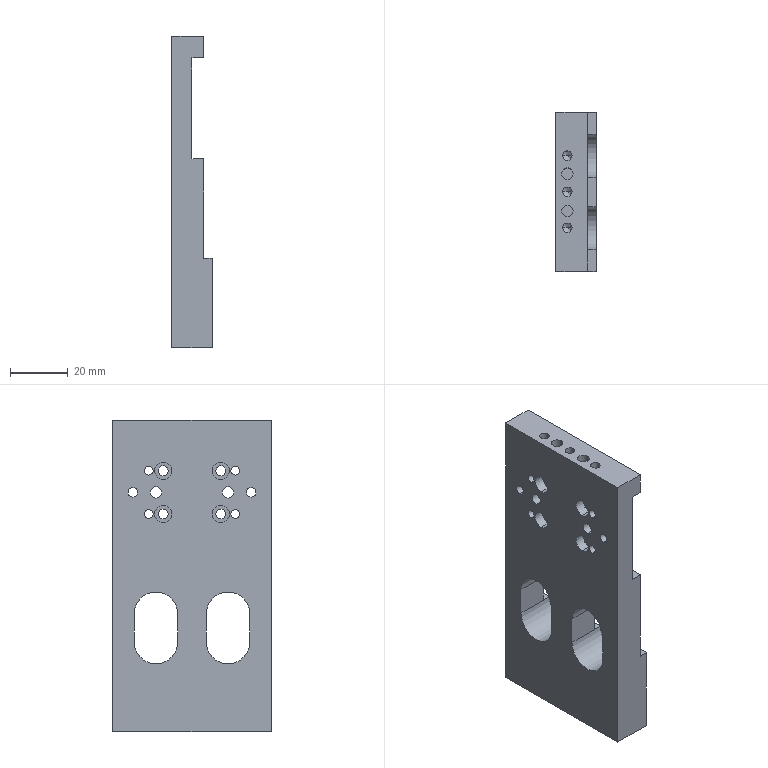Part | STEP file | 11-FG-B02311 | 1 solid | 90 faces | box 14 x 55 x 108 mm | volume 52508 mm3 | cylinder 54 | plane 26 | cone 10 | commonest cylinder face diameters 3.3 x10 3 x8 3.4 x8 4 x8 5 x8 6 x8